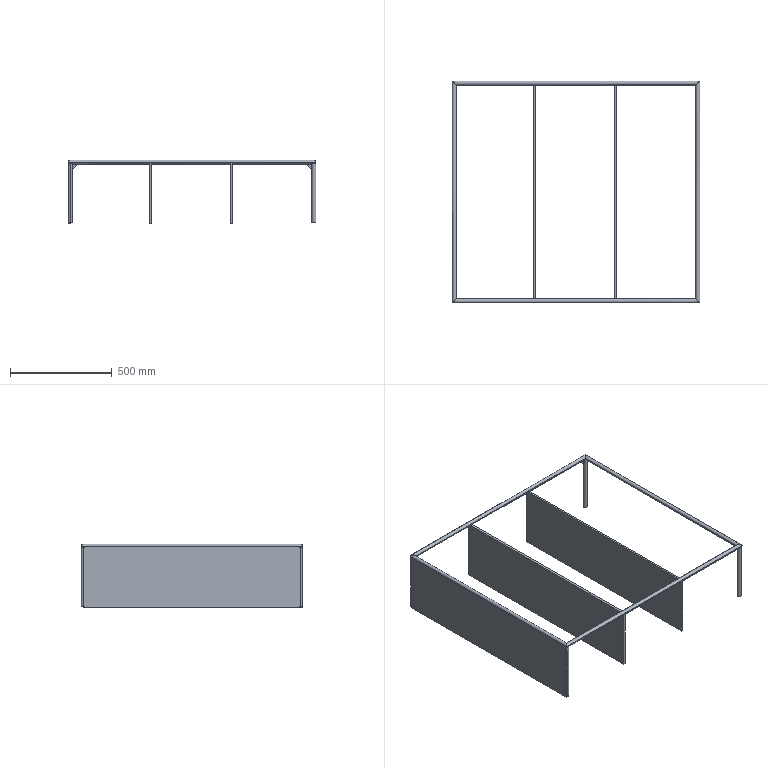Part | SolidWorks | features 3DProfileFeature 2, Gusset 2, ExtruThin 1, WeldMemberFeat 1, WeldmentFeature 1 | 13 solids | 80 faces | box 1220 x 1093 x 315 mm | volume 10289928 mm3 | plane 40 | cylinder 40 | commonest cylinder face diameters 20 x24 17.6 x16